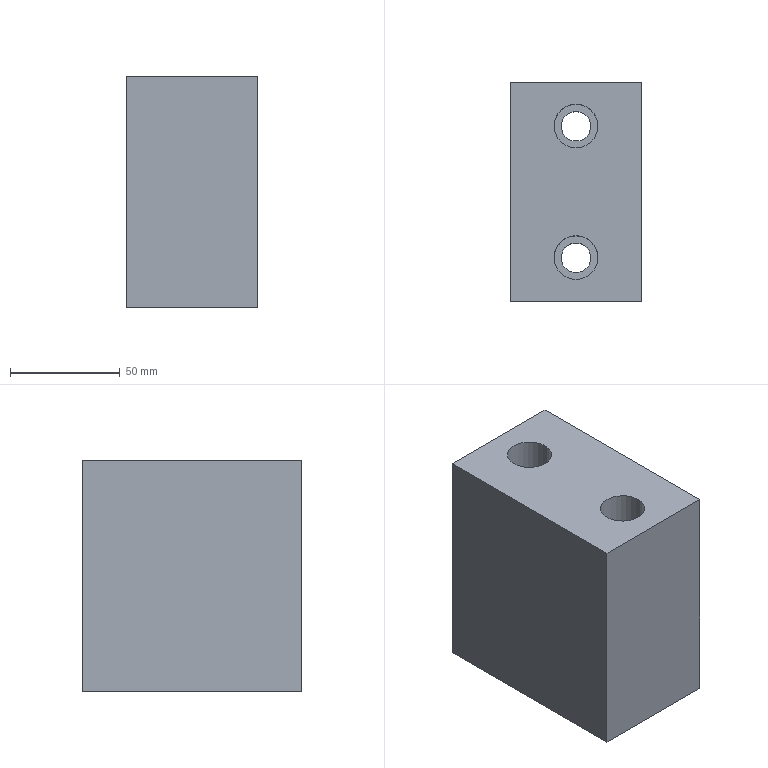Part | NX | features 28 2 | 1 solid | 12 faces | box 60 x 100 x 105.5 mm | volume 580394 mm3 | plane 8 | cylinder 4 | commonest cylinder face diameters 13.5 x2 20 x2
STEP:
#1=CARTESIAN_POINT('',(3948.25,-592.5,-73.));
#2=VERTEX_POINT('',#1);
#3=CARTESIAN_POINT('',(3955.,-592.5,-73.));
#4=DIRECTION('',(0.,0.,-1.));
#5=DIRECTION('',(-1.,0.,0.));
#6=AXIS2_PLACEMENT_3D('',#3,#4,#5);
#7=CIRCLE('',#6,6.75);
#8=EDGE_CURVE('',#2,#2,#7,.T.);
#9=ORIENTED_EDGE('',*,*,#8,.T.);
#10=EDGE_LOOP('',(#9));
#11=FACE_BOUND('',#10,.T.);
#12=CARTESIAN_POINT('',(3955.,-602.5,-73.));
#13=VERTEX_POINT('',#12);
#14=CARTESIAN_POINT('',(3955.,-592.5,-73.));
#15=DIRECTION('',(0.,0.,-1.));
#16=DIRECTION('',(0.,-1.,0.));
#17=AXIS2_PLACEMENT_3D('',#14,#15,#16);
#18=CIRCLE('',#17,10.);
#19=EDGE_CURVE('',#13,#13,#18,.T.);
#20=ORIENTED_EDGE('',*,*,#19,.F.);
#21=EDGE_LOOP('',(#20));
#22=FACE_BOUND('',#21,.T.);
#23=CARTESIAN_POINT('',(3959.241,-596.363,-73.));
#24=DIRECTION('',(0.,0.,-1.));
#25=DIRECTION('',(0.,-1.,0.));
#26=AXIS2_PLACEMENT_3D('',#23,#24,#25);
#27=PLANE('',#26);
#28=ADVANCED_FACE('',(#11,#22),#27,.F.);
#29=ORIENTED_EDGE('',*,*,#19,.T.);
#30=EDGE_LOOP('',(#29));
#31=FACE_BOUND('',#30,.T.);
#32=CARTESIAN_POINT('',(3955.,-602.5,-7.5));
#33=VERTEX_POINT('',#32);
#34=CARTESIAN_POINT('',(3955.,-592.5,-7.5));
#35=DIRECTION('',(0.,0.,1.));
#36=DIRECTION('',(0.,-1.,0.));
#37=AXIS2_PLACEMENT_3D('',#34,#35,#36);
#38=CIRCLE('',#37,10.);
#39=EDGE_CURVE('',#33,#33,#38,.T.);
#40=ORIENTED_EDGE('',*,*,#39,.T.);
#41=EDGE_LOOP('',(#40));
#42=FACE_BOUND('',#41,.T.);
#43=CARTESIAN_POINT('',(3955.,-592.5,-32.5));
#44=DIRECTION('',(0.,0.,-1.));
#45=DIRECTION('',(0.,-1.,0.));
#46=AXIS2_PLACEMENT_3D('',#43,#44,#45);
#47=CYLINDRICAL_SURFACE('',#46,10.);
#48=ADVANCED_FACE('',(#31,#42),#47,.F.);
#49=CARTESIAN_POINT('',(3948.25,-592.5,-113.));
#50=VERTEX_POINT('',#49);
#51=CARTESIAN_POINT('',(3955.,-592.5,-113.));
#52=DIRECTION('',(0.,0.,-1.));
#53=DIRECTION('',(-1.,0.,0.));
#54=AXIS2_PLACEMENT_3D('',#51,#52,#53);
#55=CIRCLE('',#54,6.75);
#56=EDGE_CURVE('',#50,#50,#55,.T.);
#57=ORIENTED_EDGE('',*,*,#56,.T.);
#58=EDGE_LOOP('',(#57));
#59=FACE_BOUND('',#58,.T.);
#60=ORIENTED_EDGE('',*,*,#8,.F.);
#61=EDGE_LOOP('',(#60));
#62=FACE_BOUND('',#61,.T.);
#63=CARTESIAN_POINT('',(3955.,-592.5,-67.5));
#64=DIRECTION('',(0.,0.,-1.));
#65=DIRECTION('',(0.,-1.,0.));
#66=AXIS2_PLACEMENT_3D('',#63,#64,#65);
#67=CYLINDRICAL_SURFACE('',#66,6.75);
#68=ADVANCED_FACE('',(#59,#62),#67,.F.);
#69=CARTESIAN_POINT('',(3948.25,-652.5,-73.));
#70=VERTEX_POINT('',#69);
#71=CARTESIAN_POINT('',(3955.,-652.5,-73.));
#72=DIRECTION('',(0.,0.,-1.));
#73=DIRECTION('',(-1.,0.,0.));
#74=AXIS2_PLACEMENT_3D('',#71,#72,#73);
#75=CIRCLE('',#74,6.75);
#76=EDGE_CURVE('',#70,#70,#75,.T.);
#77=ORIENTED_EDGE('',*,*,#76,.T.);
#78=EDGE_LOOP('',(#77));
#79=FACE_BOUND('',#78,.T.);
#80=CARTESIAN_POINT('',(3955.,-642.5,-73.));
#81=VERTEX_POINT('',#80);
#82=CARTESIAN_POINT('',(3955.,-652.5,-73.));
#83=DIRECTION('',(0.,0.,-1.));
#84=DIRECTION('',(0.,1.,0.));
#85=AXIS2_PLACEMENT_3D('',#82,#83,#84);
#86=CIRCLE('',#85,10.);
#87=EDGE_CURVE('',#81,#81,#86,.T.);
#88=ORIENTED_EDGE('',*,*,#87,.F.);
#89=EDGE_LOOP('',(#88));
#90=FACE_BOUND('',#89,.T.);
#91=CARTESIAN_POINT('',(3959.241,-648.637,-73.));
#92=DIRECTION('',(0.,0.,-1.));
#93=DIRECTION('',(0.,1.,0.));
#94=AXIS2_PLACEMENT_3D('',#91,#92,#93);
#95=PLANE('',#94);
#96=ADVANCED_FACE('',(#79,#90),#95,.F.);
#97=CARTESIAN_POINT('',(3948.25,-652.5,-113.));
#98=VERTEX_POINT('',#97);
#99=CARTESIAN_POINT('',(3955.,-652.5,-113.));
#100=DIRECTION('',(0.,0.,-1.));
#101=DIRECTION('',(-1.,0.,0.));
#102=AXIS2_PLACEMENT_3D('',#99,#100,#101);
#103=CIRCLE('',#102,6.75);
#104=EDGE_CURVE('',#98,#98,#103,.T.);
#105=ORIENTED_EDGE('',*,*,#104,.T.);
#106=EDGE_LOOP('',(#105));
#107=FACE_BOUND('',#106,.T.);
#108=ORIENTED_EDGE('',*,*,#76,.F.);
#109=EDGE_LOOP('',(#108));
#110=FACE_BOUND('',#109,.T.);
#111=CARTESIAN_POINT('',(3955.,-652.5,-67.5));
#112=DIRECTION('',(0.,0.,-1.));
#113=DIRECTION('',(0.,1.,0.));
#114=AXIS2_PLACEMENT_3D('',#111,#112,#113);
#115=CYLINDRICAL_SURFACE('',#114,6.75);
#116=ADVANCED_FACE('',(#107,#110),#115,.F.);
#117=CARTESIAN_POINT('',(3925.,-572.5,-7.5));
#118=VERTEX_POINT('',#117);
#119=CARTESIAN_POINT('',(3925.,-572.5,-113.));
#120=VERTEX_POINT('',#119);
#121=CARTESIAN_POINT('',(3925.,-572.5,-113.));
#122=DIRECTION('',(0.,0.,-1.));
#123=VECTOR('',#122,1000.);
#124=LINE('',#121,#123);
#125=EDGE_CURVE('',#118,#120,#124,.T.);
#126=ORIENTED_EDGE('',*,*,#125,.F.);
#127=CARTESIAN_POINT('',(3985.,-572.5,-7.5));
#128=VERTEX_POINT('',#127);
#129=CARTESIAN_POINT('',(3985.,-572.5,-7.5));
#130=DIRECTION('',(-1.,0.,0.));
#131=VECTOR('',#130,1000.);
#132=LINE('',#129,#131);
#133=EDGE_CURVE('',#128,#118,#132,.T.);
#134=ORIENTED_EDGE('',*,*,#133,.F.);
#135=CARTESIAN_POINT('',(3985.,-572.5,-113.));
#136=VERTEX_POINT('',#135);
#137=CARTESIAN_POINT('',(3985.,-572.5,-113.));
#138=DIRECTION('',(0.,0.,1.));
#139=VECTOR('',#138,1000.);
#140=LINE('',#137,#139);
#141=EDGE_CURVE('',#136,#128,#140,.T.);
#142=ORIENTED_EDGE('',*,*,#141,.F.);
#143=CARTESIAN_POINT('',(3985.,-572.5,-113.));
#144=DIRECTION('',(1.,0.,0.));
#145=VECTOR('',#144,1000.);
#146=LINE('',#143,#145);
#147=EDGE_CURVE('',#120,#136,#146,.T.);
#148=ORIENTED_EDGE('',*,*,#147,.F.);
#149=EDGE_LOOP('',(#126,#134,#142,#148));
#150=FACE_BOUND('',#149,.T.);
#151=CARTESIAN_POINT('',(3985.,-572.5,-113.));
#152=DIRECTION('',(0.,1.,0.));
#153=DIRECTION('',(0.,0.,1.));
#154=AXIS2_PLACEMENT_3D('',#151,#152,#153);
#155=PLANE('',#154);
#156=ADVANCED_FACE('',(#150),#155,.T.);
#157=ORIENTED_EDGE('',*,*,#141,.T.);
#158=CARTESIAN_POINT('',(3985.,-672.5,-7.5));
#159=VERTEX_POINT('',#158);
#160=CARTESIAN_POINT('',(3985.,-642.5,-7.5));
#161=DIRECTION('',(0.,1.,0.));
#162=VECTOR('',#161,1000.);
#163=LINE('',#160,#162);
#164=EDGE_CURVE('',#159,#128,#163,.T.);
#165=ORIENTED_EDGE('',*,*,#164,.F.);
#166=CARTESIAN_POINT('',(3985.,-672.5,-113.));
#167=VERTEX_POINT('',#166);
#168=CARTESIAN_POINT('',(3985.,-672.5,-113.));
#169=DIRECTION('',(0.,0.,-1.));
#170=VECTOR('',#169,1000.);
#171=LINE('',#168,#170);
#172=EDGE_CURVE('',#159,#167,#171,.T.);
#173=ORIENTED_EDGE('',*,*,#172,.T.);
#174=CARTESIAN_POINT('',(3985.,266.621,-113.));
#175=DIRECTION('',(0.,1.,0.));
#176=VECTOR('',#175,1000.);
#177=LINE('',#174,#176);
#178=EDGE_CURVE('',#167,#136,#177,.T.);
#179=ORIENTED_EDGE('',*,*,#178,.T.);
#180=EDGE_LOOP('',(#157,#165,#173,#179));
#181=FACE_BOUND('',#180,.T.);
#182=CARTESIAN_POINT('',(3985.,-642.5,-113.));
#183=DIRECTION('',(1.,0.,0.));
#184=DIRECTION('',(0.,0.,1.));
#185=AXIS2_PLACEMENT_3D('',#182,#183,#184);
#186=PLANE('',#185);
#187=ADVANCED_FACE('',(#181),#186,.T.);
#188=ORIENTED_EDGE('',*,*,#172,.F.);
#189=CARTESIAN_POINT('',(3925.,-672.5,-7.5));
#190=VERTEX_POINT('',#189);
#191=CARTESIAN_POINT('',(3985.,-672.5,-7.5));
#192=DIRECTION('',(1.,0.,0.));
#193=VECTOR('',#192,1000.);
#194=LINE('',#191,#193);
#195=EDGE_CURVE('',#190,#159,#194,.T.);
#196=ORIENTED_EDGE('',*,*,#195,.F.);
#197=CARTESIAN_POINT('',(3925.,-672.5,-113.));
#198=VERTEX_POINT('',#197);
#199=CARTESIAN_POINT('',(3925.,-672.5,-113.));
#200=DIRECTION('',(0.,0.,1.));
#201=VECTOR('',#200,1000.);
#202=LINE('',#199,#201);
#203=EDGE_CURVE('',#198,#190,#202,.T.);
#204=ORIENTED_EDGE('',*,*,#203,.F.);
#205=CARTESIAN_POINT('',(3600.,-672.5,-113.));
#206=DIRECTION('',(1.,0.,0.));
#207=VECTOR('',#206,1000.);
#208=LINE('',#205,#207);
#209=EDGE_CURVE('',#198,#167,#208,.T.);
#210=ORIENTED_EDGE('',*,*,#209,.T.);
#211=EDGE_LOOP('',(#188,#196,#204,#210));
#212=FACE_BOUND('',#211,.T.);
#213=CARTESIAN_POINT('',(3985.,-672.5,-113.));
#214=DIRECTION('',(0.,-1.,0.));
#215=DIRECTION('',(0.,0.,-1.));
#216=AXIS2_PLACEMENT_3D('',#213,#214,#215);
#217=PLANE('',#216);
#218=ADVANCED_FACE('',(#212),#217,.T.);
#219=ORIENTED_EDGE('',*,*,#203,.T.);
#220=CARTESIAN_POINT('',(3925.,-642.5,-7.5));
#221=DIRECTION('',(0.,-1.,0.));
#222=VECTOR('',#221,1000.);
#223=LINE('',#220,#222);
#224=EDGE_CURVE('',#118,#190,#223,.T.);
#225=ORIENTED_EDGE('',*,*,#224,.F.);
#226=ORIENTED_EDGE('',*,*,#125,.T.);
#227=CARTESIAN_POINT('',(3925.,266.621,-113.));
#228=DIRECTION('',(0.,-1.,0.));
#229=VECTOR('',#228,1000.);
#230=LINE('',#227,#229);
#231=EDGE_CURVE('',#120,#198,#230,.T.);
#232=ORIENTED_EDGE('',*,*,#231,.T.);
#233=EDGE_LOOP('',(#219,#225,#226,#232));
#234=FACE_BOUND('',#233,.T.);
#235=CARTESIAN_POINT('',(3925.,-642.5,-113.));
#236=DIRECTION('',(-1.,0.,0.));
#237=DIRECTION('',(0.,0.,-1.));
#238=AXIS2_PLACEMENT_3D('',#235,#236,#237);
#239=PLANE('',#238);
#240=ADVANCED_FACE('',(#234),#239,.T.);
#241=ORIENTED_EDGE('',*,*,#87,.T.);
#242=EDGE_LOOP('',(#241));
#243=FACE_BOUND('',#242,.T.);
#244=CARTESIAN_POINT('',(3955.,-642.5,-7.5));
#245=VERTEX_POINT('',#244);
#246=CARTESIAN_POINT('',(3955.,-652.5,-7.5));
#247=DIRECTION('',(0.,0.,1.));
#248=DIRECTION('',(0.,1.,0.));
#249=AXIS2_PLACEMENT_3D('',#246,#247,#248);
#250=CIRCLE('',#249,10.);
#251=EDGE_CURVE('',#245,#245,#250,.T.);
#252=ORIENTED_EDGE('',*,*,#251,.T.);
#253=EDGE_LOOP('',(#252));
#254=FACE_BOUND('',#253,.T.);
#255=CARTESIAN_POINT('',(3955.,-652.5,-32.5));
#256=DIRECTION('',(0.,0.,-1.));
#257=DIRECTION('',(0.,1.,0.));
#258=AXIS2_PLACEMENT_3D('',#255,#256,#257);
#259=CYLINDRICAL_SURFACE('',#258,10.);
#260=ADVANCED_FACE('',(#243,#254),#259,.F.);
#261=ORIENTED_EDGE('',*,*,#39,.F.);
#262=EDGE_LOOP('',(#261));
#263=FACE_BOUND('',#262,.T.);
#264=ORIENTED_EDGE('',*,*,#251,.F.);
#265=EDGE_LOOP('',(#264));
#266=FACE_BOUND('',#265,.T.);
#267=ORIENTED_EDGE('',*,*,#224,.T.);
#268=ORIENTED_EDGE('',*,*,#195,.T.);
#269=ORIENTED_EDGE('',*,*,#164,.T.);
#270=ORIENTED_EDGE('',*,*,#133,.T.);
#271=EDGE_LOOP('',(#267,#268,#269,#270));
#272=FACE_BOUND('',#271,.T.);
#273=CARTESIAN_POINT('',(3985.,-572.5,-7.5));
#274=DIRECTION('',(0.,0.,1.));
#275=DIRECTION('',(0.,-1.,0.));
#276=AXIS2_PLACEMENT_3D('',#273,#274,#275);
#277=PLANE('',#276);
#278=ADVANCED_FACE('',(#263,#266,#272),#277,.T.);
#279=ORIENTED_EDGE('',*,*,#56,.F.);
#280=EDGE_LOOP('',(#279));
#281=FACE_BOUND('',#280,.T.);
#282=ORIENTED_EDGE('',*,*,#209,.F.);
#283=ORIENTED_EDGE('',*,*,#231,.F.);
#284=ORIENTED_EDGE('',*,*,#147,.T.);
#285=ORIENTED_EDGE('',*,*,#178,.F.);
#286=EDGE_LOOP('',(#282,#283,#284,#285));
#287=FACE_BOUND('',#286,.T.);
#288=ORIENTED_EDGE('',*,*,#104,.F.);
#289=EDGE_LOOP('',(#288));
#290=FACE_BOUND('',#289,.T.);
#291=CARTESIAN_POINT('',(3600.,266.621,-113.));
#292=DIRECTION('',(0.,0.,-1.));
#293=DIRECTION('',(0.,1.,0.));
#294=AXIS2_PLACEMENT_3D('',#291,#292,#293);
#295=PLANE('',#294);
#296=ADVANCED_FACE('',(#281,#287,#290),#295,.T.);
#297=CLOSED_SHELL('',(#28,#48,#68,#96,#116,#156,#187,#218,#240,#260,#278,#296));
#298=MANIFOLD_SOLID_BREP('',#297);
#299=(LENGTH_UNIT()NAMED_UNIT(*)SI_UNIT(.MILLI.,.METRE.));
#300=UNCERTAINTY_MEASURE_WITH_UNIT(LENGTH_MEASURE(0.00001),#299,'','');
#301=(NAMED_UNIT(*)PLANE_ANGLE_UNIT()SI_UNIT($,.RADIAN.));
#302=(NAMED_UNIT(*)SI_UNIT($,.STERADIAN.)SOLID_ANGLE_UNIT());
#303=(GEOMETRIC_REPRESENTATION_CONTEXT(3)GLOBAL_UNCERTAINTY_ASSIGNED_CONTEXT((#300))GLOBAL_UNIT_ASSIGNED_CONTEXT((#299,#301,#302))REPRESENTATION_CONTEXT('',''));
#304=ADVANCED_BREP_SHAPE_REPRESENTATION('',(#298),#303);